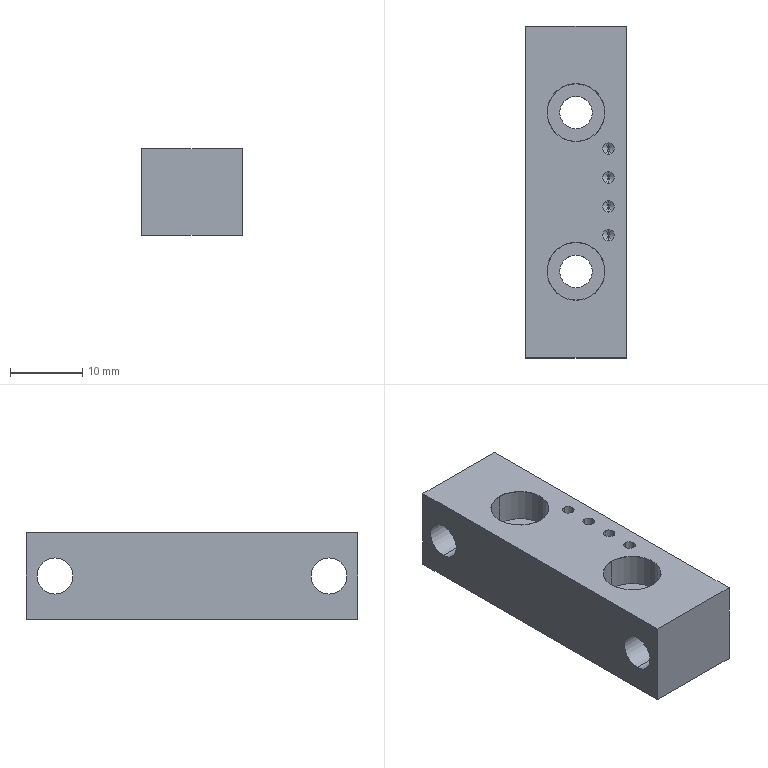Part | NX | features M2 螺纹孔1 2 | 1 solid | 40 faces | box 14 x 46 x 12 mm | volume 6437 mm3 | cylinder 20 | cone 12 | plane 8 | commonest cylinder face diameters 1.6 x8 4.5 x4 5 x4 8 x4
STEP:
#1=CARTESIAN_POINT('',(-56.5,97.8,-87.7));
#2=VERTEX_POINT('',#1);
#3=CARTESIAN_POINT('',(-56.5,96.2,-87.7));
#4=VERTEX_POINT('',#3);
#5=CARTESIAN_POINT('',(-56.5,97.,-87.7));
#6=DIRECTION('',(0.,0.,1.));
#7=DIRECTION('',(0.,-1.,0.));
#8=AXIS2_PLACEMENT_3D('',#5,#6,#7);
#9=CIRCLE('',#8,0.8);
#10=EDGE_CURVE('',#2,#4,#9,.T.);
#11=ORIENTED_EDGE('',*,*,#10,.F.);
#12=CARTESIAN_POINT('',(-56.5,97.8,-82.5));
#13=VERTEX_POINT('',#12);
#14=CARTESIAN_POINT('',(-56.5,97.8,-82.5));
#15=DIRECTION('',(0.,0.,1.));
#16=VECTOR('',#15,1000.);
#17=LINE('',#14,#16);
#18=EDGE_CURVE('',#2,#13,#17,.T.);
#19=ORIENTED_EDGE('',*,*,#18,.T.);
#20=CARTESIAN_POINT('',(-56.5,96.2,-82.5));
#21=VERTEX_POINT('',#20);
#22=CARTESIAN_POINT('',(-56.5,97.,-82.5));
#23=DIRECTION('',(0.,0.,1.));
#24=DIRECTION('',(0.,-1.,0.));
#25=AXIS2_PLACEMENT_3D('',#22,#23,#24);
#26=CIRCLE('',#25,0.8);
#27=EDGE_CURVE('',#13,#21,#26,.T.);
#28=ORIENTED_EDGE('',*,*,#27,.T.);
#29=CARTESIAN_POINT('',(-56.5,96.2,-82.5));
#30=DIRECTION('',(0.,0.,1.));
#31=VECTOR('',#30,1000.);
#32=LINE('',#29,#31);
#33=EDGE_CURVE('',#21,#4,#32,.F.);
#34=ORIENTED_EDGE('',*,*,#33,.T.);
#35=EDGE_LOOP('',(#11,#19,#28,#34));
#36=FACE_BOUND('',#35,.T.);
#37=CARTESIAN_POINT('',(-56.5,97.,-82.5));
#38=DIRECTION('',(0.,0.,1.));
#39=DIRECTION('',(0.,1.,0.));
#40=AXIS2_PLACEMENT_3D('',#37,#38,#39);
#41=CYLINDRICAL_SURFACE('',#40,0.8);
#42=ADVANCED_FACE('',(#36),#41,.F.);
#43=CARTESIAN_POINT('',(-56.5,97.,-88.181));
#44=VERTEX_POINT('',#43);
#45=CARTESIAN_POINT('',(-56.5,96.2,-87.7));
#46=DIRECTION('',(0.,-0.8572,0.515));
#47=VECTOR('',#46,1000.);
#48=LINE('',#45,#47);
#49=EDGE_CURVE('',#4,#44,#48,.F.);
#50=ORIENTED_EDGE('',*,*,#49,.T.);
#51=CARTESIAN_POINT('',(-56.5,97.8,-87.7));
#52=DIRECTION('',(0.,0.8572,0.515));
#53=VECTOR('',#52,1000.);
#54=LINE('',#51,#53);
#55=EDGE_CURVE('',#44,#2,#54,.T.);
#56=ORIENTED_EDGE('',*,*,#55,.T.);
#57=ORIENTED_EDGE('',*,*,#10,.T.);
#58=EDGE_LOOP('',(#50,#56,#57));
#59=FACE_BOUND('',#58,.T.);
#60=CARTESIAN_POINT('',(-56.5,97.,-87.7));
#61=DIRECTION('',(0.,0.,1.));
#62=DIRECTION('',(0.,1.,0.));
#63=AXIS2_PLACEMENT_3D('',#60,#61,#62);
#64=CONICAL_SURFACE('',#63,0.8,1.03);
#65=ADVANCED_FACE('',(#59),#64,.F.);
#66=CARTESIAN_POINT('',(-56.5,93.8,-87.7));
#67=VERTEX_POINT('',#66);
#68=CARTESIAN_POINT('',(-56.5,92.2,-87.7));
#69=VERTEX_POINT('',#68);
#70=CARTESIAN_POINT('',(-56.5,93.,-87.7));
#71=DIRECTION('',(0.,0.,1.));
#72=DIRECTION('',(0.,-1.,0.));
#73=AXIS2_PLACEMENT_3D('',#70,#71,#72);
#74=CIRCLE('',#73,0.8);
#75=EDGE_CURVE('',#67,#69,#74,.T.);
#76=ORIENTED_EDGE('',*,*,#75,.F.);
#77=CARTESIAN_POINT('',(-56.5,93.8,-82.5));
#78=VERTEX_POINT('',#77);
#79=CARTESIAN_POINT('',(-56.5,93.8,-82.5));
#80=DIRECTION('',(0.,0.,1.));
#81=VECTOR('',#80,1000.);
#82=LINE('',#79,#81);
#83=EDGE_CURVE('',#67,#78,#82,.T.);
#84=ORIENTED_EDGE('',*,*,#83,.T.);
#85=CARTESIAN_POINT('',(-56.5,92.2,-82.5));
#86=VERTEX_POINT('',#85);
#87=CARTESIAN_POINT('',(-56.5,93.,-82.5));
#88=DIRECTION('',(0.,0.,1.));
#89=DIRECTION('',(0.,-1.,0.));
#90=AXIS2_PLACEMENT_3D('',#87,#88,#89);
#91=CIRCLE('',#90,0.8);
#92=EDGE_CURVE('',#78,#86,#91,.T.);
#93=ORIENTED_EDGE('',*,*,#92,.T.);
#94=CARTESIAN_POINT('',(-56.5,92.2,-82.5));
#95=DIRECTION('',(0.,0.,1.));
#96=VECTOR('',#95,1000.);
#97=LINE('',#94,#96);
#98=EDGE_CURVE('',#86,#69,#97,.F.);
#99=ORIENTED_EDGE('',*,*,#98,.T.);
#100=EDGE_LOOP('',(#76,#84,#93,#99));
#101=FACE_BOUND('',#100,.T.);
#102=CARTESIAN_POINT('',(-56.5,93.,-82.5));
#103=DIRECTION('',(0.,0.,1.));
#104=DIRECTION('',(0.,1.,0.));
#105=AXIS2_PLACEMENT_3D('',#102,#103,#104);
#106=CYLINDRICAL_SURFACE('',#105,0.8);
#107=ADVANCED_FACE('',(#101),#106,.F.);
#108=CARTESIAN_POINT('',(-56.5,93.,-88.181));
#109=VERTEX_POINT('',#108);
#110=CARTESIAN_POINT('',(-56.5,92.2,-87.7));
#111=DIRECTION('',(0.,-0.8572,0.515));
#112=VECTOR('',#111,1000.);
#113=LINE('',#110,#112);
#114=EDGE_CURVE('',#109,#69,#113,.T.);
#115=ORIENTED_EDGE('',*,*,#114,.F.);
#116=CARTESIAN_POINT('',(-56.5,93.8,-87.7));
#117=DIRECTION('',(0.,0.8572,0.515));
#118=VECTOR('',#117,1000.);
#119=LINE('',#116,#118);
#120=EDGE_CURVE('',#67,#109,#119,.F.);
#121=ORIENTED_EDGE('',*,*,#120,.F.);
#122=ORIENTED_EDGE('',*,*,#75,.T.);
#123=EDGE_LOOP('',(#115,#121,#122));
#124=FACE_BOUND('',#123,.T.);
#125=CARTESIAN_POINT('',(-56.5,93.,-87.7));
#126=DIRECTION('',(0.,0.,1.));
#127=DIRECTION('',(0.,1.,0.));
#128=AXIS2_PLACEMENT_3D('',#125,#126,#127);
#129=CONICAL_SURFACE('',#128,0.8,1.03);
#130=ADVANCED_FACE('',(#124),#129,.F.);
#131=CARTESIAN_POINT('',(-56.5,105.8,-87.7));
#132=VERTEX_POINT('',#131);
#133=CARTESIAN_POINT('',(-56.5,104.2,-87.7));
#134=VERTEX_POINT('',#133);
#135=CARTESIAN_POINT('',(-56.5,105.,-87.7));
#136=DIRECTION('',(0.,0.,1.));
#137=DIRECTION('',(0.,-1.,0.));
#138=AXIS2_PLACEMENT_3D('',#135,#136,#137);
#139=CIRCLE('',#138,0.8);
#140=EDGE_CURVE('',#132,#134,#139,.T.);
#141=ORIENTED_EDGE('',*,*,#140,.F.);
#142=CARTESIAN_POINT('',(-56.5,105.8,-82.5));
#143=VERTEX_POINT('',#142);
#144=CARTESIAN_POINT('',(-56.5,105.8,-82.5));
#145=DIRECTION('',(0.,0.,1.));
#146=VECTOR('',#145,1000.);
#147=LINE('',#144,#146);
#148=EDGE_CURVE('',#143,#132,#147,.F.);
#149=ORIENTED_EDGE('',*,*,#148,.F.);
#150=CARTESIAN_POINT('',(-56.5,104.2,-82.5));
#151=VERTEX_POINT('',#150);
#152=CARTESIAN_POINT('',(-56.5,105.,-82.5));
#153=DIRECTION('',(0.,0.,1.));
#154=DIRECTION('',(0.,-1.,0.));
#155=AXIS2_PLACEMENT_3D('',#152,#153,#154);
#156=CIRCLE('',#155,0.8);
#157=EDGE_CURVE('',#143,#151,#156,.T.);
#158=ORIENTED_EDGE('',*,*,#157,.T.);
#159=CARTESIAN_POINT('',(-56.5,104.2,-82.5));
#160=DIRECTION('',(0.,0.,1.));
#161=VECTOR('',#160,1000.);
#162=LINE('',#159,#161);
#163=EDGE_CURVE('',#134,#151,#162,.T.);
#164=ORIENTED_EDGE('',*,*,#163,.F.);
#165=EDGE_LOOP('',(#141,#149,#158,#164));
#166=FACE_BOUND('',#165,.T.);
#167=CARTESIAN_POINT('',(-56.5,105.,-82.5));
#168=DIRECTION('',(0.,0.,1.));
#169=DIRECTION('',(0.,1.,0.));
#170=AXIS2_PLACEMENT_3D('',#167,#168,#169);
#171=CYLINDRICAL_SURFACE('',#170,0.8);
#172=ADVANCED_FACE('',(#166),#171,.F.);
#173=CARTESIAN_POINT('',(-56.5,105.,-88.181));
#174=VERTEX_POINT('',#173);
#175=CARTESIAN_POINT('',(-56.5,104.2,-87.7));
#176=DIRECTION('',(0.,-0.8572,0.515));
#177=VECTOR('',#176,1000.);
#178=LINE('',#175,#177);
#179=EDGE_CURVE('',#174,#134,#178,.T.);
#180=ORIENTED_EDGE('',*,*,#179,.F.);
#181=CARTESIAN_POINT('',(-56.5,105.8,-87.7));
#182=DIRECTION('',(0.,0.8572,0.515));
#183=VECTOR('',#182,1000.);
#184=LINE('',#181,#183);
#185=EDGE_CURVE('',#132,#174,#184,.F.);
#186=ORIENTED_EDGE('',*,*,#185,.F.);
#187=ORIENTED_EDGE('',*,*,#140,.T.);
#188=EDGE_LOOP('',(#180,#186,#187));
#189=FACE_BOUND('',#188,.T.);
#190=CARTESIAN_POINT('',(-56.5,105.,-87.7));
#191=DIRECTION('',(0.,0.,1.));
#192=DIRECTION('',(0.,1.,0.));
#193=AXIS2_PLACEMENT_3D('',#190,#191,#192);
#194=CONICAL_SURFACE('',#193,0.8,1.03);
#195=ADVANCED_FACE('',(#189),#194,.F.);
#196=CARTESIAN_POINT('',(-56.5,101.8,-87.7));
#197=VERTEX_POINT('',#196);
#198=CARTESIAN_POINT('',(-56.5,100.2,-87.7));
#199=VERTEX_POINT('',#198);
#200=CARTESIAN_POINT('',(-56.5,101.,-87.7));
#201=DIRECTION('',(0.,0.,1.));
#202=DIRECTION('',(0.,-1.,0.));
#203=AXIS2_PLACEMENT_3D('',#200,#201,#202);
#204=CIRCLE('',#203,0.8);
#205=EDGE_CURVE('',#197,#199,#204,.T.);
#206=ORIENTED_EDGE('',*,*,#205,.F.);
#207=CARTESIAN_POINT('',(-56.5,101.8,-82.5));
#208=VERTEX_POINT('',#207);
#209=CARTESIAN_POINT('',(-56.5,101.8,-82.5));
#210=DIRECTION('',(0.,0.,1.));
#211=VECTOR('',#210,1000.);
#212=LINE('',#209,#211);
#213=EDGE_CURVE('',#197,#208,#212,.T.);
#214=ORIENTED_EDGE('',*,*,#213,.T.);
#215=CARTESIAN_POINT('',(-56.5,100.2,-82.5));
#216=VERTEX_POINT('',#215);
#217=CARTESIAN_POINT('',(-56.5,101.,-82.5));
#218=DIRECTION('',(0.,0.,1.));
#219=DIRECTION('',(0.,-1.,0.));
#220=AXIS2_PLACEMENT_3D('',#217,#218,#219);
#221=CIRCLE('',#220,0.8);
#222=EDGE_CURVE('',#208,#216,#221,.T.);
#223=ORIENTED_EDGE('',*,*,#222,.T.);
#224=CARTESIAN_POINT('',(-56.5,100.2,-82.5));
#225=DIRECTION('',(0.,0.,1.));
#226=VECTOR('',#225,1000.);
#227=LINE('',#224,#226);
#228=EDGE_CURVE('',#216,#199,#227,.F.);
#229=ORIENTED_EDGE('',*,*,#228,.T.);
#230=EDGE_LOOP('',(#206,#214,#223,#229));
#231=FACE_BOUND('',#230,.T.);
#232=CARTESIAN_POINT('',(-56.5,101.,-82.5));
#233=DIRECTION('',(0.,0.,1.));
#234=DIRECTION('',(0.,1.,0.));
#235=AXIS2_PLACEMENT_3D('',#232,#233,#234);
#236=CYLINDRICAL_SURFACE('',#235,0.8);
#237=ADVANCED_FACE('',(#231),#236,.F.);
#238=CARTESIAN_POINT('',(-56.5,101.,-88.181));
#239=VERTEX_POINT('',#238);
#240=CARTESIAN_POINT('',(-56.5,100.2,-87.7));
#241=DIRECTION('',(0.,-0.8572,0.515));
#242=VECTOR('',#241,1000.);
#243=LINE('',#240,#242);
#244=EDGE_CURVE('',#199,#239,#243,.F.);
#245=ORIENTED_EDGE('',*,*,#244,.T.);
#246=CARTESIAN_POINT('',(-56.5,101.8,-87.7));
#247=DIRECTION('',(0.,0.8572,0.515));
#248=VECTOR('',#247,1000.);
#249=LINE('',#246,#248);
#250=EDGE_CURVE('',#239,#197,#249,.T.);
#251=ORIENTED_EDGE('',*,*,#250,.T.);
#252=ORIENTED_EDGE('',*,*,#205,.T.);
#253=EDGE_LOOP('',(#245,#251,#252));
#254=FACE_BOUND('',#253,.T.);
#255=CARTESIAN_POINT('',(-56.5,101.,-87.7));
#256=DIRECTION('',(0.,0.,1.));
#257=DIRECTION('',(0.,1.,0.));
#258=AXIS2_PLACEMENT_3D('',#255,#256,#257);
#259=CONICAL_SURFACE('',#258,0.8,1.03);
#260=ADVANCED_FACE('',(#254),#259,.F.);
#261=CARTESIAN_POINT('',(-54.,80.,-86.));
#262=VERTEX_POINT('',#261);
#263=CARTESIAN_POINT('',(-54.,80.,-91.));
#264=VERTEX_POINT('',#263);
#265=CARTESIAN_POINT('',(-54.,80.,-88.5));
#266=DIRECTION('',(-1.,0.,0.));
#267=DIRECTION('',(0.,0.,-1.));
#268=AXIS2_PLACEMENT_3D('',#265,#266,#267);
#269=CIRCLE('',#268,2.5);
#270=EDGE_CURVE('',#262,#264,#269,.T.);
#271=ORIENTED_EDGE('',*,*,#270,.F.);
#272=CARTESIAN_POINT('',(-68.,80.,-86.));
#273=VERTEX_POINT('',#272);
#274=CARTESIAN_POINT('',(-68.,80.,-86.));
#275=DIRECTION('',(-1.,0.,0.));
#276=VECTOR('',#275,1000.);
#277=LINE('',#274,#276);
#278=EDGE_CURVE('',#262,#273,#277,.T.);
#279=ORIENTED_EDGE('',*,*,#278,.T.);
#280=CARTESIAN_POINT('',(-68.,80.,-91.));
#281=VERTEX_POINT('',#280);
#282=CARTESIAN_POINT('',(-68.,80.,-88.5));
#283=DIRECTION('',(-1.,0.,0.));
#284=DIRECTION('',(0.,0.,-1.));
#285=AXIS2_PLACEMENT_3D('',#282,#283,#284);
#286=CIRCLE('',#285,2.5);
#287=EDGE_CURVE('',#273,#281,#286,.T.);
#288=ORIENTED_EDGE('',*,*,#287,.T.);
#289=CARTESIAN_POINT('',(-68.,80.,-91.));
#290=DIRECTION('',(-1.,0.,0.));
#291=VECTOR('',#290,1000.);
#292=LINE('',#289,#291);
#293=EDGE_CURVE('',#281,#264,#292,.F.);
#294=ORIENTED_EDGE('',*,*,#293,.T.);
#295=EDGE_LOOP('',(#271,#279,#288,#294));
#296=FACE_BOUND('',#295,.T.);
#297=CARTESIAN_POINT('',(-68.,80.,-88.5));
#298=DIRECTION('',(-1.,0.,0.));
#299=DIRECTION('',(0.,0.,1.));
#300=AXIS2_PLACEMENT_3D('',#297,#298,#299);
#301=CYLINDRICAL_SURFACE('',#300,2.5);
#302=ADVANCED_FACE('',(#296),#301,.F.);
#303=CARTESIAN_POINT('',(-54.,118.,-86.));
#304=VERTEX_POINT('',#303);
#305=CARTESIAN_POINT('',(-54.,118.,-91.));
#306=VERTEX_POINT('',#305);
#307=CARTESIAN_POINT('',(-54.,118.,-88.5));
#308=DIRECTION('',(-1.,0.,0.));
#309=DIRECTION('',(0.,0.,-1.));
#310=AXIS2_PLACEMENT_3D('',#307,#308,#309);
#311=CIRCLE('',#310,2.5);
#312=EDGE_CURVE('',#304,#306,#311,.T.);
#313=ORIENTED_EDGE('',*,*,#312,.F.);
#314=CARTESIAN_POINT('',(-68.,118.,-86.));
#315=VERTEX_POINT('',#314);
#316=CARTESIAN_POINT('',(-68.,118.,-86.));
#317=DIRECTION('',(-1.,0.,0.));
#318=VECTOR('',#317,1000.);
#319=LINE('',#316,#318);
#320=EDGE_CURVE('',#304,#315,#319,.T.);
#321=ORIENTED_EDGE('',*,*,#320,.T.);
#322=CARTESIAN_POINT('',(-68.,118.,-91.));
#323=VERTEX_POINT('',#322);
#324=CARTESIAN_POINT('',(-68.,118.,-88.5));
#325=DIRECTION('',(-1.,0.,0.));
#326=DIRECTION('',(0.,0.,-1.));
#327=AXIS2_PLACEMENT_3D('',#324,#325,#326);
#328=CIRCLE('',#327,2.5);
#329=EDGE_CURVE('',#315,#323,#328,.T.);
#330=ORIENTED_EDGE('',*,*,#329,.T.);
#331=CARTESIAN_POINT('',(-68.,118.,-91.));
#332=DIRECTION('',(-1.,0.,0.));
#333=VECTOR('',#332,1000.);
#334=LINE('',#331,#333);
#335=EDGE_CURVE('',#323,#306,#334,.F.);
#336=ORIENTED_EDGE('',*,*,#335,.T.);
#337=EDGE_LOOP('',(#313,#321,#330,#336));
#338=FACE_BOUND('',#337,.T.);
#339=CARTESIAN_POINT('',(-68.,118.,-88.5));
#340=DIRECTION('',(-1.,0.,0.));
#341=DIRECTION('',(0.,0.,1.));
#342=AXIS2_PLACEMENT_3D('',#339,#340,#341);
#343=CYLINDRICAL_SURFACE('',#342,2.5);
#344=ADVANCED_FACE('',(#338),#343,.F.);
#345=CARTESIAN_POINT('',(-61.,92.,-82.525));
#346=VERTEX_POINT('',#345);
#347=CARTESIAN_POINT('',(-61.,84.,-82.525));
#348=VERTEX_POINT('',#347);
#349=CARTESIAN_POINT('',(-61.,88.,-82.525));
#350=DIRECTION('',(0.,0.,1.));
#351=DIRECTION('',(0.,-1.,0.));
#352=AXIS2_PLACEMENT_3D('',#349,#350,#351);
#353=CIRCLE('',#352,4.);
#354=EDGE_CURVE('',#346,#348,#353,.T.);
#355=ORIENTED_EDGE('',*,*,#354,.F.);
#356=CARTESIAN_POINT('',(-61.,92.025,-82.5));
#357=VERTEX_POINT('',#356);
#358=CARTESIAN_POINT('',(-61.,92.025,-82.5));
#359=DIRECTION('',(0.,0.7071,0.7071));
#360=VECTOR('',#359,1000.);
#361=LINE('',#358,#360);
#362=EDGE_CURVE('',#346,#357,#361,.T.);
#363=ORIENTED_EDGE('',*,*,#362,.T.);
#364=CARTESIAN_POINT('',(-61.,83.975,-82.5));
#365=VERTEX_POINT('',#364);
#366=CARTESIAN_POINT('',(-61.,88.,-82.5));
#367=DIRECTION('',(0.,0.,1.));
#368=DIRECTION('',(0.,-1.,0.));
#369=AXIS2_PLACEMENT_3D('',#366,#367,#368);
#370=CIRCLE('',#369,4.025);
#371=EDGE_CURVE('',#357,#365,#370,.T.);
#372=ORIENTED_EDGE('',*,*,#371,.T.);
#373=CARTESIAN_POINT('',(-61.,83.975,-82.5));
#374=DIRECTION('',(0.,-0.7071,0.7071));
#375=VECTOR('',#374,1000.);
#376=LINE('',#373,#375);
#377=EDGE_CURVE('',#365,#348,#376,.F.);
#378=ORIENTED_EDGE('',*,*,#377,.T.);
#379=EDGE_LOOP('',(#355,#363,#372,#378));
#380=FACE_BOUND('',#379,.T.);
#381=CARTESIAN_POINT('',(-61.,88.,-82.5));
#382=DIRECTION('',(0.,0.,1.));
#383=DIRECTION('',(0.,1.,0.));
#384=AXIS2_PLACEMENT_3D('',#381,#382,#383);
#385=CONICAL_SURFACE('',#384,4.025,0.7854);
#386=ADVANCED_FACE('',(#380),#385,.F.);
#387=CARTESIAN_POINT('',(-61.,92.,-87.1));
#388=VERTEX_POINT('',#387);
#389=CARTESIAN_POINT('',(-61.,84.,-87.1));
#390=VERTEX_POINT('',#389);
#391=CARTESIAN_POINT('',(-61.,88.,-87.1));
#392=DIRECTION('',(0.,0.,1.));
#393=DIRECTION('',(0.,-1.,0.));
#394=AXIS2_PLACEMENT_3D('',#391,#392,#393);
#395=CIRCLE('',#394,4.);
#396=EDGE_CURVE('',#388,#390,#395,.T.);
#397=ORIENTED_EDGE('',*,*,#396,.F.);
#398=CARTESIAN_POINT('',(-61.,92.,-82.5));
#399=DIRECTION('',(0.,0.,1.));
#400=VECTOR('',#399,1000.);
#401=LINE('',#398,#400);
#402=EDGE_CURVE('',#388,#346,#401,.T.);
#403=ORIENTED_EDGE('',*,*,#402,.T.);
#404=ORIENTED_EDGE('',*,*,#354,.T.);
#405=CARTESIAN_POINT('',(-61.,84.,-82.5));
#406=DIRECTION('',(0.,0.,1.));
#407=VECTOR('',#406,1000.);
#408=LINE('',#405,#407);
#409=EDGE_CURVE('',#348,#390,#408,.F.);
#410=ORIENTED_EDGE('',*,*,#409,.T.);
#411=EDGE_LOOP('',(#397,#403,#404,#410));
#412=FACE_BOUND('',#411,.T.);
#413=CARTESIAN_POINT('',(-61.,88.,-82.5));
#414=DIRECTION('',(0.,0.,1.));
#415=DIRECTION('',(0.,1.,0.));
#416=AXIS2_PLACEMENT_3D('',#413,#414,#415);
#417=CYLINDRICAL_SURFACE('',#416,4.);
#418=ADVANCED_FACE('',(#412),#417,.F.);
#419=CARTESIAN_POINT('',(-61.,90.25,-94.5));
#420=VERTEX_POINT('',#419);
#421=CARTESIAN_POINT('',(-61.,85.75,-94.5));
#422=VERTEX_POINT('',#421);
#423=CARTESIAN_POINT('',(-61.,88.,-94.5));
#424=DIRECTION('',(0.,0.,1.));
#425=DIRECTION('',(0.,-1.,0.));
#426=AXIS2_PLACEMENT_3D('',#423,#424,#425);
#427=CIRCLE('',#426,2.25);
#428=EDGE_CURVE('',#420,#422,#427,.T.);
#429=ORIENTED_EDGE('',*,*,#428,.F.);
#430=CARTESIAN_POINT('',(-61.,90.25,-87.1));
#431=VERTEX_POINT('',#430);
#432=CARTESIAN_POINT('',(-61.,90.25,-82.5));
#433=DIRECTION('',(0.,0.,1.));
#434=VECTOR('',#433,1000.);
#435=LINE('',#432,#434);
#436=EDGE_CURVE('',#431,#420,#435,.F.);
#437=ORIENTED_EDGE('',*,*,#436,.F.);
#438=CARTESIAN_POINT('',(-61.,85.75,-87.1));
#439=VERTEX_POINT('',#438);
#440=CARTESIAN_POINT('',(-61.,88.,-87.1));
#441=DIRECTION('',(0.,0.,1.));
#442=DIRECTION('',(0.,-1.,0.));
#443=AXIS2_PLACEMENT_3D('',#440,#441,#442);
#444=CIRCLE('',#443,2.25);
#445=EDGE_CURVE('',#431,#439,#444,.T.);
#446=ORIENTED_EDGE('',*,*,#445,.T.);
#447=CARTESIAN_POINT('',(-61.,85.75,-82.5));
#448=DIRECTION('',(0.,0.,1.));
#449=VECTOR('',#448,1000.);
#450=LINE('',#447,#449);
#451=EDGE_CURVE('',#422,#439,#450,.T.);
#452=ORIENTED_EDGE('',*,*,#451,.F.);
#453=EDGE_LOOP('',(#429,#437,#446,#452));
#454=FACE_BOUND('',#453,.T.);
#455=CARTESIAN_POINT('',(-61.,88.,-82.5));
#456=DIRECTION('',(0.,0.,1.));
#457=DIRECTION('',(0.,1.,0.));
#458=AXIS2_PLACEMENT_3D('',#455,#456,#457);
#459=CYLINDRICAL_SURFACE('',#458,2.25);
#460=ADVANCED_FACE('',(#454),#459,.F.);
#461=CARTESIAN_POINT('',(-61.,114.,-82.525));
#462=VERTEX_POINT('',#461);
#463=CARTESIAN_POINT('',(-61.,106.,-82.525));
#464=VERTEX_POINT('',#463);
#465=CARTESIAN_POINT('',(-61.,110.,-82.525));
#466=DIRECTION('',(0.,0.,1.));
#467=DIRECTION('',(0.,-1.,0.));
#468=AXIS2_PLACEMENT_3D('',#465,#466,#467);
#469=CIRCLE('',#468,4.);
#470=EDGE_CURVE('',#462,#464,#469,.T.);
#471=ORIENTED_EDGE('',*,*,#470,.F.);
#472=CARTESIAN_POINT('',(-61.,114.025,-82.5));
#473=VERTEX_POINT('',#472);
#474=CARTESIAN_POINT('',(-61.,114.025,-82.5));
#475=DIRECTION('',(0.,0.7071,0.7071));
#476=VECTOR('',#475,1000.);
#477=LINE('',#474,#476);
#478=EDGE_CURVE('',#473,#462,#477,.F.);
#479=ORIENTED_EDGE('',*,*,#478,.F.);
#480=CARTESIAN_POINT('',(-61.,105.975,-82.5));
#481=VERTEX_POINT('',#480);
#482=CARTESIAN_POINT('',(-61.,110.,-82.5));
#483=DIRECTION('',(0.,0.,1.));
#484=DIRECTION('',(0.,-1.,0.));
#485=AXIS2_PLACEMENT_3D('',#482,#483,#484);
#486=CIRCLE('',#485,4.025);
#487=EDGE_CURVE('',#473,#481,#486,.T.);
#488=ORIENTED_EDGE('',*,*,#487,.T.);
#489=CARTESIAN_POINT('',(-61.,105.975,-82.5));
#490=DIRECTION('',(0.,-0.7071,0.7071));
#491=VECTOR('',#490,1000.);
#492=LINE('',#489,#491);
#493=EDGE_CURVE('',#464,#481,#492,.T.);
#494=ORIENTED_EDGE('',*,*,#493,.F.);
#495=EDGE_LOOP('',(#471,#479,#488,#494));
#496=FACE_BOUND('',#495,.T.);
#497=CARTESIAN_POINT('',(-61.,110.,-82.5));
#498=DIRECTION('',(0.,0.,1.));
#499=DIRECTION('',(0.,1.,0.));
#500=AXIS2_PLACEMENT_3D('',#497,#498,#499);
#501=CONICAL_SURFACE('',#500,4.025,0.7854);
#502=ADVANCED_FACE('',(#496),#501,.F.);
#503=CARTESIAN_POINT('',(-61.,114.,-87.1));
#504=VERTEX_POINT('',#503);
#505=CARTESIAN_POINT('',(-61.,106.,-87.1));
#506=VERTEX_POINT('',#505);
#507=CARTESIAN_POINT('',(-61.,110.,-87.1));
#508=DIRECTION('',(0.,0.,1.));
#509=DIRECTION('',(0.,-1.,0.));
#510=AXIS2_PLACEMENT_3D('',#507,#508,#509);
#511=CIRCLE('',#510,4.);
#512=EDGE_CURVE('',#504,#506,#511,.T.);
#513=ORIENTED_EDGE('',*,*,#512,.F.);
#514=CARTESIAN_POINT('',(-61.,114.,-82.5));
#515=DIRECTION('',(0.,0.,1.));
#516=VECTOR('',#515,1000.);
#517=LINE('',#514,#516);
#518=EDGE_CURVE('',#462,#504,#517,.F.);
#519=ORIENTED_EDGE('',*,*,#518,.F.);
#520=ORIENTED_EDGE('',*,*,#470,.T.);
#521=CARTESIAN_POINT('',(-61.,106.,-82.5));
#522=DIRECTION('',(0.,0.,1.));
#523=VECTOR('',#522,1000.);
#524=LINE('',#521,#523);
#525=EDGE_CURVE('',#506,#464,#524,.T.);
#526=ORIENTED_EDGE('',*,*,#525,.F.);
#527=EDGE_LOOP('',(#513,#519,#520,#526));
#528=FACE_BOUND('',#527,.T.);
#529=CARTESIAN_POINT('',(-61.,110.,-82.5));
#530=DIRECTION('',(0.,0.,1.));
#531=DIRECTION('',(0.,1.,0.));
#532=AXIS2_PLACEMENT_3D('',#529,#530,#531);
#533=CYLINDRICAL_SURFACE('',#532,4.);
#534=ADVANCED_FACE('',(#528),#533,.F.);
#535=CARTESIAN_POINT('',(-61.,112.25,-94.5));
#536=VERTEX_POINT('',#535);
#537=CARTESIAN_POINT('',(-61.,107.75,-94.5));
#538=VERTEX_POINT('',#537);
#539=CARTESIAN_POINT('',(-61.,110.,-94.5));
#540=DIRECTION('',(0.,0.,1.));
#541=DIRECTION('',(0.,-1.,0.));
#542=AXIS2_PLACEMENT_3D('',#539,#540,#541);
#543=CIRCLE('',#542,2.25);
#544=EDGE_CURVE('',#536,#538,#543,.T.);
#545=ORIENTED_EDGE('',*,*,#544,.F.);
#546=CARTESIAN_POINT('',(-61.,112.25,-87.1));
#547=VERTEX_POINT('',#546);
#548=CARTESIAN_POINT('',(-61.,112.25,-82.5));
#549=DIRECTION('',(0.,0.,1.));
#550=VECTOR('',#549,1000.);
#551=LINE('',#548,#550);
#552=EDGE_CURVE('',#536,#547,#551,.T.);
#553=ORIENTED_EDGE('',*,*,#552,.T.);
#554=CARTESIAN_POINT('',(-61.,107.75,-87.1));
#555=VERTEX_POINT('',#554);
#556=CARTESIAN_POINT('',(-61.,110.,-87.1));
#557=DIRECTION('',(0.,0.,1.));
#558=DIRECTION('',(0.,-1.,0.));
#559=AXIS2_PLACEMENT_3D('',#556,#557,#558);
#560=CIRCLE('',#559,2.25);
#561=EDGE_CURVE('',#547,#555,#560,.T.);
#562=ORIENTED_EDGE('',*,*,#561,.T.);
#563=CARTESIAN_POINT('',(-61.,107.75,-82.5));
#564=DIRECTION('',(0.,0.,1.));
#565=VECTOR('',#564,1000.);
#566=LINE('',#563,#565);
#567=EDGE_CURVE('',#555,#538,#566,.F.);
#568=ORIENTED_EDGE('',*,*,#567,.T.);
#569=EDGE_LOOP('',(#545,#553,#562,#568));
#570=FACE_BOUND('',#569,.T.);
#571=CARTESIAN_POINT('',(-61.,110.,-82.5));
#572=DIRECTION('',(0.,0.,1.));
#573=DIRECTION('',(0.,1.,0.));
#574=AXIS2_PLACEMENT_3D('',#571,#572,#573);
#575=CYLINDRICAL_SURFACE('',#574,2.25);
#576=ADVANCED_FACE('',(#570),#575,.F.);
#577=CARTESIAN_POINT('',(-68.,76.,-94.5));
#578=VERTEX_POINT('',#577);
#579=CARTESIAN_POINT('',(-54.,76.,-94.5));
#580=VERTEX_POINT('',#579);
#581=CARTESIAN_POINT('',(-54.,76.,-94.5));
#582=DIRECTION('',(1.,0.,0.));
#583=VECTOR('',#582,1000.);
#584=LINE('',#581,#583);
#585=EDGE_CURVE('',#578,#580,#584,.T.);
#586=ORIENTED_EDGE('',*,*,#585,.T.);
#587=CARTESIAN_POINT('',(-54.,76.,-82.5));
#588=VERTEX_POINT('',#587);
#589=CARTESIAN_POINT('',(-54.,76.,-82.5));
#590=DIRECTION('',(0.,0.,-1.));
#591=VECTOR('',#590,1000.);
#592=LINE('',#589,#591);
#593=EDGE_CURVE('',#588,#580,#592,.T.);
#594=ORIENTED_EDGE('',*,*,#593,.F.);
#595=CARTESIAN_POINT('',(-68.,76.,-82.5));
#596=VERTEX_POINT('',#595);
#597=CARTESIAN_POINT('',(-54.,76.,-82.5));
#598=DIRECTION('',(1.,0.,0.));
#599=VECTOR('',#598,1000.);
#600=LINE('',#597,#599);
#601=EDGE_CURVE('',#596,#588,#600,.T.);
#602=ORIENTED_EDGE('',*,*,#601,.F.);
#603=CARTESIAN_POINT('',(-68.,76.,-82.5));
#604=DIRECTION('',(0.,0.,-1.));
#605=VECTOR('',#604,1000.);
#606=LINE('',#603,#605);
#607=EDGE_CURVE('',#596,#578,#606,.T.);
#608=ORIENTED_EDGE('',*,*,#607,.T.);
#609=EDGE_LOOP('',(#586,#594,#602,#608));
#610=FACE_BOUND('',#609,.T.);
#611=CARTESIAN_POINT('',(-54.,76.,-82.5));
#612=DIRECTION('',(0.,1.,0.));
#613=DIRECTION('',(0.,0.,-1.));
#614=AXIS2_PLACEMENT_3D('',#611,#612,#613);
#615=PLANE('',#614);
#616=ADVANCED_FACE('',(#610),#615,.F.);
#617=CARTESIAN_POINT('',(-54.,80.,-88.5));
#618=DIRECTION('',(-1.,0.,0.));
#619=DIRECTION('',(0.,0.,-1.));
#620=AXIS2_PLACEMENT_3D('',#617,#618,#619);
#621=CIRCLE('',#620,2.5);
#622=EDGE_CURVE('',#264,#262,#621,.T.);
#623=ORIENTED_EDGE('',*,*,#622,.T.);
#624=ORIENTED_EDGE('',*,*,#270,.T.);
#625=EDGE_LOOP('',(#623,#624));
#626=FACE_BOUND('',#625,.T.);
#627=CARTESIAN_POINT('',(-54.,118.,-88.5));
#628=DIRECTION('',(-1.,0.,0.));
#629=DIRECTION('',(0.,0.,-1.));
#630=AXIS2_PLACEMENT_3D('',#627,#628,#629);
#631=CIRCLE('',#630,2.5);
#632=EDGE_CURVE('',#306,#304,#631,.T.);
#633=ORIENTED_EDGE('',*,*,#632,.T.);
#634=ORIENTED_EDGE('',*,*,#312,.T.);
#635=EDGE_LOOP('',(#633,#634));
#636=FACE_BOUND('',#635,.T.);
#637=CARTESIAN_POINT('',(-54.,122.,-94.5));
#638=VERTEX_POINT('',#637);
#639=CARTESIAN_POINT('',(-54.,122.,-94.5));
#640=DIRECTION('',(0.,1.,0.));
#641=VECTOR('',#640,1000.);
#642=LINE('',#639,#641);
#643=EDGE_CURVE('',#580,#638,#642,.T.);
#644=ORIENTED_EDGE('',*,*,#643,.T.);
#645=CARTESIAN_POINT('',(-54.,122.,-82.5));
#646=VERTEX_POINT('',#645);
#647=CARTESIAN_POINT('',(-54.,122.,-82.5));
#648=DIRECTION('',(0.,0.,-1.));
#649=VECTOR('',#648,1000.);
#650=LINE('',#647,#649);
#651=EDGE_CURVE('',#646,#638,#650,.T.);
#652=ORIENTED_EDGE('',*,*,#651,.F.);
#653=CARTESIAN_POINT('',(-54.,122.,-82.5));
#654=DIRECTION('',(0.,1.,0.));
#655=VECTOR('',#654,1000.);
#656=LINE('',#653,#655);
#657=EDGE_CURVE('',#588,#646,#656,.T.);
#658=ORIENTED_EDGE('',*,*,#657,.F.);
#659=ORIENTED_EDGE('',*,*,#593,.T.);
#660=EDGE_LOOP('',(#644,#652,#658,#659));
#661=FACE_BOUND('',#660,.T.);
#662=CARTESIAN_POINT('',(-54.,122.,-82.5));
#663=DIRECTION('',(-1.,0.,0.));
#664=DIRECTION('',(0.,0.,1.));
#665=AXIS2_PLACEMENT_3D('',#662,#663,#664);
#666=PLANE('',#665);
#667=ADVANCED_FACE('',(#626,#636,#661),#666,.F.);
#668=CARTESIAN_POINT('',(-68.,122.,-94.5));
#669=VERTEX_POINT('',#668);
#670=CARTESIAN_POINT('',(-54.,122.,-94.5));
#671=DIRECTION('',(-1.,0.,0.));
#672=VECTOR('',#671,1000.);
#673=LINE('',#670,#672);
#674=EDGE_CURVE('',#638,#669,#673,.T.);
#675=ORIENTED_EDGE('',*,*,#674,.T.);
#676=CARTESIAN_POINT('',(-68.,122.,-82.5));
#677=VERTEX_POINT('',#676);
#678=CARTESIAN_POINT('',(-68.,122.,-82.5));
#679=DIRECTION('',(0.,0.,-1.));
#680=VECTOR('',#679,1000.);
#681=LINE('',#678,#680);
#682=EDGE_CURVE('',#677,#669,#681,.T.);
#683=ORIENTED_EDGE('',*,*,#682,.F.);
#684=CARTESIAN_POINT('',(-54.,122.,-82.5));
#685=DIRECTION('',(-1.,0.,0.));
#686=VECTOR('',#685,1000.);
#687=LINE('',#684,#686);
#688=EDGE_CURVE('',#646,#677,#687,.T.);
#689=ORIENTED_EDGE('',*,*,#688,.F.);
#690=ORIENTED_EDGE('',*,*,#651,.T.);
#691=EDGE_LOOP('',(#675,#683,#689,#690));
#692=FACE_BOUND('',#691,.T.);
#693=CARTESIAN_POINT('',(-54.,122.,-82.5));
#694=DIRECTION('',(0.,-1.,0.));
#695=DIRECTION('',(0.,0.,1.));
#696=AXIS2_PLACEMENT_3D('',#693,#694,#695);
#697=PLANE('',#696);
#698=ADVANCED_FACE('',(#692),#697,.F.);
#699=CARTESIAN_POINT('',(-68.,80.,-88.5));
#700=DIRECTION('',(-1.,0.,0.));
#701=DIRECTION('',(0.,0.,-1.));
#702=AXIS2_PLACEMENT_3D('',#699,#700,#701);
#703=CIRCLE('',#702,2.5);
#704=EDGE_CURVE('',#281,#273,#703,.T.);
#705=ORIENTED_EDGE('',*,*,#704,.F.);
#706=ORIENTED_EDGE('',*,*,#287,.F.);
#707=EDGE_LOOP('',(#705,#706));
#708=FACE_BOUND('',#707,.T.);
#709=CARTESIAN_POINT('',(-68.,118.,-88.5));
#710=DIRECTION('',(-1.,0.,0.));
#711=DIRECTION('',(0.,0.,-1.));
#712=AXIS2_PLACEMENT_3D('',#709,#710,#711);
#713=CIRCLE('',#712,2.5);
#714=EDGE_CURVE('',#323,#315,#713,.T.);
#715=ORIENTED_EDGE('',*,*,#714,.F.);
#716=ORIENTED_EDGE('',*,*,#329,.F.);
#717=EDGE_LOOP('',(#715,#716));
#718=FACE_BOUND('',#717,.T.);
#719=CARTESIAN_POINT('',(-68.,122.,-94.5));
#720=DIRECTION('',(0.,-1.,0.));
#721=VECTOR('',#720,1000.);
#722=LINE('',#719,#721);
#723=EDGE_CURVE('',#669,#578,#722,.T.);
#724=ORIENTED_EDGE('',*,*,#723,.T.);
#725=ORIENTED_EDGE('',*,*,#607,.F.);
#726=CARTESIAN_POINT('',(-68.,122.,-82.5));
#727=DIRECTION('',(0.,-1.,0.));
#728=VECTOR('',#727,1000.);
#729=LINE('',#726,#728);
#730=EDGE_CURVE('',#677,#596,#729,.T.);
#731=ORIENTED_EDGE('',*,*,#730,.F.);
#732=ORIENTED_EDGE('',*,*,#682,.T.);
#733=EDGE_LOOP('',(#724,#725,#731,#732));
#734=FACE_BOUND('',#733,.T.);
#735=CARTESIAN_POINT('',(-68.,122.,-82.5));
#736=DIRECTION('',(1.,0.,0.));
#737=DIRECTION('',(0.,0.,-1.));
#738=AXIS2_PLACEMENT_3D('',#735,#736,#737);
#739=PLANE('',#738);
#740=ADVANCED_FACE('',(#708,#718,#734),#739,.F.);
#741=CARTESIAN_POINT('',(-56.5,97.,-82.5));
#742=DIRECTION('',(0.,0.,1.));
#743=DIRECTION('',(0.,-1.,0.));
#744=AXIS2_PLACEMENT_3D('',#741,#742,#743);
#745=CIRCLE('',#744,0.8);
#746=EDGE_CURVE('',#21,#13,#745,.T.);
#747=ORIENTED_EDGE('',*,*,#746,.F.);
#748=ORIENTED_EDGE('',*,*,#27,.F.);
#749=EDGE_LOOP('',(#747,#748));
#750=FACE_BOUND('',#749,.T.);
#751=CARTESIAN_POINT('',(-56.5,93.,-82.5));
#752=DIRECTION('',(0.,0.,1.));
#753=DIRECTION('',(0.,-1.,0.));
#754=AXIS2_PLACEMENT_3D('',#751,#752,#753);
#755=CIRCLE('',#754,0.8);
#756=EDGE_CURVE('',#86,#78,#755,.T.);
#757=ORIENTED_EDGE('',*,*,#756,.F.);
#758=ORIENTED_EDGE('',*,*,#92,.F.);
#759=EDGE_LOOP('',(#757,#758));
#760=FACE_BOUND('',#759,.T.);
#761=CARTESIAN_POINT('',(-56.5,105.,-82.5));
#762=DIRECTION('',(0.,0.,1.));
#763=DIRECTION('',(0.,-1.,0.));
#764=AXIS2_PLACEMENT_3D('',#761,#762,#763);
#765=CIRCLE('',#764,0.8);
#766=EDGE_CURVE('',#151,#143,#765,.T.);
#767=ORIENTED_EDGE('',*,*,#766,.F.);
#768=ORIENTED_EDGE('',*,*,#157,.F.);
#769=EDGE_LOOP('',(#767,#768));
#770=FACE_BOUND('',#769,.T.);
#771=CARTESIAN_POINT('',(-56.5,101.,-82.5));
#772=DIRECTION('',(0.,0.,1.));
#773=DIRECTION('',(0.,-1.,0.));
#774=AXIS2_PLACEMENT_3D('',#771,#772,#773);
#775=CIRCLE('',#774,0.8);
#776=EDGE_CURVE('',#216,#208,#775,.T.);
#777=ORIENTED_EDGE('',*,*,#776,.F.);
#778=ORIENTED_EDGE('',*,*,#222,.F.);
#779=EDGE_LOOP('',(#777,#778));
#780=FACE_BOUND('',#779,.T.);
#781=CARTESIAN_POINT('',(-61.,88.,-82.5));
#782=DIRECTION('',(0.,0.,1.));
#783=DIRECTION('',(0.,-1.,0.));
#784=AXIS2_PLACEMENT_3D('',#781,#782,#783);
#785=CIRCLE('',#784,4.025);
#786=EDGE_CURVE('',#365,#357,#785,.T.);
#787=ORIENTED_EDGE('',*,*,#786,.F.);
#788=ORIENTED_EDGE('',*,*,#371,.F.);
#789=EDGE_LOOP('',(#787,#788));
#790=FACE_BOUND('',#789,.T.);
#791=CARTESIAN_POINT('',(-61.,110.,-82.5));
#792=DIRECTION('',(0.,0.,1.));
#793=DIRECTION('',(0.,-1.,0.));
#794=AXIS2_PLACEMENT_3D('',#791,#792,#793);
#795=CIRCLE('',#794,4.025);
#796=EDGE_CURVE('',#481,#473,#795,.T.);
#797=ORIENTED_EDGE('',*,*,#796,.F.);
#798=ORIENTED_EDGE('',*,*,#487,.F.);
#799=EDGE_LOOP('',(#797,#798));
#800=FACE_BOUND('',#799,.T.);
#801=ORIENTED_EDGE('',*,*,#601,.T.);
#802=ORIENTED_EDGE('',*,*,#657,.T.);
#803=ORIENTED_EDGE('',*,*,#688,.T.);
#804=ORIENTED_EDGE('',*,*,#730,.T.);
#805=EDGE_LOOP('',(#801,#802,#803,#804));
#806=FACE_BOUND('',#805,.T.);
#807=CARTESIAN_POINT('',(-61.,99.,-82.5));
#808=DIRECTION('',(0.,0.,1.));
#809=DIRECTION('',(0.,1.,0.));
#810=AXIS2_PLACEMENT_3D('',#807,#808,#809);
#811=PLANE('',#810);
#812=ADVANCED_FACE('',(#750,#760,#770,#780,#790,#800,#806),#811,.T.);
#813=CARTESIAN_POINT('',(-61.,88.,-94.5));
#814=DIRECTION('',(0.,0.,1.));
#815=DIRECTION('',(0.,-1.,0.));
#816=AXIS2_PLACEMENT_3D('',#813,#814,#815);
#817=CIRCLE('',#816,2.25);
#818=EDGE_CURVE('',#422,#420,#817,.T.);
#819=ORIENTED_EDGE('',*,*,#818,.T.);
#820=ORIENTED_EDGE('',*,*,#428,.T.);
#821=EDGE_LOOP('',(#819,#820));
#822=FACE_BOUND('',#821,.T.);
#823=CARTESIAN_POINT('',(-61.,110.,-94.5));
#824=DIRECTION('',(0.,0.,1.));
#825=DIRECTION('',(0.,-1.,0.));
#826=AXIS2_PLACEMENT_3D('',#823,#824,#825);
#827=CIRCLE('',#826,2.25);
#828=EDGE_CURVE('',#538,#536,#827,.T.);
#829=ORIENTED_EDGE('',*,*,#828,.T.);
#830=ORIENTED_EDGE('',*,*,#544,.T.);
#831=EDGE_LOOP('',(#829,#830));
#832=FACE_BOUND('',#831,.T.);
#833=ORIENTED_EDGE('',*,*,#585,.F.);
#834=ORIENTED_EDGE('',*,*,#723,.F.);
#835=ORIENTED_EDGE('',*,*,#674,.F.);
#836=ORIENTED_EDGE('',*,*,#643,.F.);
#837=EDGE_LOOP('',(#833,#834,#835,#836));
#838=FACE_BOUND('',#837,.T.);
#839=CARTESIAN_POINT('',(-61.,99.,-94.5));
#840=DIRECTION('',(0.,0.,1.));
#841=DIRECTION('',(0.,1.,0.));
#842=AXIS2_PLACEMENT_3D('',#839,#840,#841);
#843=PLANE('',#842);
#844=ADVANCED_FACE('',(#822,#832,#838),#843,.F.);
#845=ORIENTED_EDGE('',*,*,#552,.F.);
#846=ORIENTED_EDGE('',*,*,#828,.F.);
#847=ORIENTED_EDGE('',*,*,#567,.F.);
#848=CARTESIAN_POINT('',(-61.,110.,-87.1));
#849=DIRECTION('',(0.,0.,1.));
#850=DIRECTION('',(0.,-1.,0.));
#851=AXIS2_PLACEMENT_3D('',#848,#849,#850);
#852=CIRCLE('',#851,2.25);
#853=EDGE_CURVE('',#555,#547,#852,.T.);
#854=ORIENTED_EDGE('',*,*,#853,.T.);
#855=EDGE_LOOP('',(#845,#846,#847,#854));
#856=FACE_BOUND('',#855,.T.);
#857=CARTESIAN_POINT('',(-61.,110.,-82.5));
#858=DIRECTION('',(0.,0.,1.));
#859=DIRECTION('',(0.,1.,0.));
#860=AXIS2_PLACEMENT_3D('',#857,#858,#859);
#861=CYLINDRICAL_SURFACE('',#860,2.25);
#862=ADVANCED_FACE('',(#856),#861,.F.);
#863=ORIENTED_EDGE('',*,*,#853,.F.);
#864=ORIENTED_EDGE('',*,*,#561,.F.);
#865=EDGE_LOOP('',(#863,#864));
#866=FACE_BOUND('',#865,.T.);
#867=CARTESIAN_POINT('',(-61.,110.,-87.1));
#868=DIRECTION('',(0.,0.,1.));
#869=DIRECTION('',(0.,-1.,0.));
#870=AXIS2_PLACEMENT_3D('',#867,#868,#869);
#871=CIRCLE('',#870,4.);
#872=EDGE_CURVE('',#506,#504,#871,.T.);
#873=ORIENTED_EDGE('',*,*,#872,.T.);
#874=ORIENTED_EDGE('',*,*,#512,.T.);
#875=EDGE_LOOP('',(#873,#874));
#876=FACE_BOUND('',#875,.T.);
#877=CARTESIAN_POINT('',(-61.,106.,-87.1));
#878=DIRECTION('',(0.,0.,-1.));
#879=DIRECTION('',(0.,-1.,0.));
#880=AXIS2_PLACEMENT_3D('',#877,#878,#879);
#881=PLANE('',#880);
#882=ADVANCED_FACE('',(#866,#876),#881,.F.);
#883=ORIENTED_EDGE('',*,*,#518,.T.);
#884=ORIENTED_EDGE('',*,*,#872,.F.);
#885=ORIENTED_EDGE('',*,*,#525,.T.);
#886=CARTESIAN_POINT('',(-61.,110.,-82.525));
#887=DIRECTION('',(0.,0.,1.));
#888=DIRECTION('',(0.,-1.,0.));
#889=AXIS2_PLACEMENT_3D('',#886,#887,#888);
#890=CIRCLE('',#889,4.);
#891=EDGE_CURVE('',#464,#462,#890,.T.);
#892=ORIENTED_EDGE('',*,*,#891,.T.);
#893=EDGE_LOOP('',(#883,#884,#885,#892));
#894=FACE_BOUND('',#893,.T.);
#895=CARTESIAN_POINT('',(-61.,110.,-82.5));
#896=DIRECTION('',(0.,0.,1.));
#897=DIRECTION('',(0.,1.,0.));
#898=AXIS2_PLACEMENT_3D('',#895,#896,#897);
#899=CYLINDRICAL_SURFACE('',#898,4.);
#900=ADVANCED_FACE('',(#894),#899,.F.);
#901=ORIENTED_EDGE('',*,*,#478,.T.);
#902=ORIENTED_EDGE('',*,*,#891,.F.);
#903=ORIENTED_EDGE('',*,*,#493,.T.);
#904=ORIENTED_EDGE('',*,*,#796,.T.);
#905=EDGE_LOOP('',(#901,#902,#903,#904));
#906=FACE_BOUND('',#905,.T.);
#907=CARTESIAN_POINT('',(-61.,110.,-82.5));
#908=DIRECTION('',(0.,0.,1.));
#909=DIRECTION('',(0.,1.,0.));
#910=AXIS2_PLACEMENT_3D('',#907,#908,#909);
#911=CONICAL_SURFACE('',#910,4.025,0.7854);
#912=ADVANCED_FACE('',(#906),#911,.F.);
#913=ORIENTED_EDGE('',*,*,#436,.T.);
#914=ORIENTED_EDGE('',*,*,#818,.F.);
#915=ORIENTED_EDGE('',*,*,#451,.T.);
#916=CARTESIAN_POINT('',(-61.,88.,-87.1));
#917=DIRECTION('',(0.,0.,1.));
#918=DIRECTION('',(0.,-1.,0.));
#919=AXIS2_PLACEMENT_3D('',#916,#917,#918);
#920=CIRCLE('',#919,2.25);
#921=EDGE_CURVE('',#439,#431,#920,.T.);
#922=ORIENTED_EDGE('',*,*,#921,.T.);
#923=EDGE_LOOP('',(#913,#914,#915,#922));
#924=FACE_BOUND('',#923,.T.);
#925=CARTESIAN_POINT('',(-61.,88.,-82.5));
#926=DIRECTION('',(0.,0.,1.));
#927=DIRECTION('',(0.,1.,0.));
#928=AXIS2_PLACEMENT_3D('',#925,#926,#927);
#929=CYLINDRICAL_SURFACE('',#928,2.25);
#930=ADVANCED_FACE('',(#924),#929,.F.);
#931=ORIENTED_EDGE('',*,*,#921,.F.);
#932=ORIENTED_EDGE('',*,*,#445,.F.);
#933=EDGE_LOOP('',(#931,#932));
#934=FACE_BOUND('',#933,.T.);
#935=CARTESIAN_POINT('',(-61.,88.,-87.1));
#936=DIRECTION('',(0.,0.,1.));
#937=DIRECTION('',(0.,-1.,0.));
#938=AXIS2_PLACEMENT_3D('',#935,#936,#937);
#939=CIRCLE('',#938,4.);
#940=EDGE_CURVE('',#390,#388,#939,.T.);
#941=ORIENTED_EDGE('',*,*,#940,.T.);
#942=ORIENTED_EDGE('',*,*,#396,.T.);
#943=EDGE_LOOP('',(#941,#942));
#944=FACE_BOUND('',#943,.T.);
#945=CARTESIAN_POINT('',(-61.,84.,-87.1));
#946=DIRECTION('',(0.,0.,-1.));
#947=DIRECTION('',(0.,-1.,0.));
#948=AXIS2_PLACEMENT_3D('',#945,#946,#947);
#949=PLANE('',#948);
#950=ADVANCED_FACE('',(#934,#944),#949,.F.);
#951=ORIENTED_EDGE('',*,*,#402,.F.);
#952=ORIENTED_EDGE('',*,*,#940,.F.);
#953=ORIENTED_EDGE('',*,*,#409,.F.);
#954=CARTESIAN_POINT('',(-61.,88.,-82.525));
#955=DIRECTION('',(0.,0.,1.));
#956=DIRECTION('',(0.,-1.,0.));
#957=AXIS2_PLACEMENT_3D('',#954,#955,#956);
#958=CIRCLE('',#957,4.);
#959=EDGE_CURVE('',#348,#346,#958,.T.);
#960=ORIENTED_EDGE('',*,*,#959,.T.);
#961=EDGE_LOOP('',(#951,#952,#953,#960));
#962=FACE_BOUND('',#961,.T.);
#963=CARTESIAN_POINT('',(-61.,88.,-82.5));
#964=DIRECTION('',(0.,0.,1.));
#965=DIRECTION('',(0.,1.,0.));
#966=AXIS2_PLACEMENT_3D('',#963,#964,#965);
#967=CYLINDRICAL_SURFACE('',#966,4.);
#968=ADVANCED_FACE('',(#962),#967,.F.);
#969=ORIENTED_EDGE('',*,*,#362,.F.);
#970=ORIENTED_EDGE('',*,*,#959,.F.);
#971=ORIENTED_EDGE('',*,*,#377,.F.);
#972=ORIENTED_EDGE('',*,*,#786,.T.);
#973=EDGE_LOOP('',(#969,#970,#971,#972));
#974=FACE_BOUND('',#973,.T.);
#975=CARTESIAN_POINT('',(-61.,88.,-82.5));
#976=DIRECTION('',(0.,0.,1.));
#977=DIRECTION('',(0.,1.,0.));
#978=AXIS2_PLACEMENT_3D('',#975,#976,#977);
#979=CONICAL_SURFACE('',#978,4.025,0.7854);
#980=ADVANCED_FACE('',(#974),#979,.F.);
#981=ORIENTED_EDGE('',*,*,#320,.F.);
#982=ORIENTED_EDGE('',*,*,#632,.F.);
#983=ORIENTED_EDGE('',*,*,#335,.F.);
#984=ORIENTED_EDGE('',*,*,#714,.T.);
#985=EDGE_LOOP('',(#981,#982,#983,#984));
#986=FACE_BOUND('',#985,.T.);
#987=CARTESIAN_POINT('',(-68.,118.,-88.5));
#988=DIRECTION('',(-1.,0.,0.));
#989=DIRECTION('',(0.,0.,1.));
#990=AXIS2_PLACEMENT_3D('',#987,#988,#989);
#991=CYLINDRICAL_SURFACE('',#990,2.5);
#992=ADVANCED_FACE('',(#986),#991,.F.);
#993=ORIENTED_EDGE('',*,*,#278,.F.);
#994=ORIENTED_EDGE('',*,*,#622,.F.);
#995=ORIENTED_EDGE('',*,*,#293,.F.);
#996=ORIENTED_EDGE('',*,*,#704,.T.);
#997=EDGE_LOOP('',(#993,#994,#995,#996));
#998=FACE_BOUND('',#997,.T.);
#999=CARTESIAN_POINT('',(-68.,80.,-88.5));
#1000=DIRECTION('',(-1.,0.,0.));
#1001=DIRECTION('',(0.,0.,1.));
#1002=AXIS2_PLACEMENT_3D('',#999,#1000,#1001);
#1003=CYLINDRICAL_SURFACE('',#1002,2.5);
#1004=ADVANCED_FACE('',(#998),#1003,.F.);
#1005=ORIENTED_EDGE('',*,*,#250,.F.);
#1006=ORIENTED_EDGE('',*,*,#244,.F.);
#1007=CARTESIAN_POINT('',(-56.5,101.,-87.7));
#1008=DIRECTION('',(0.,0.,1.));
#1009=DIRECTION('',(0.,-1.,0.));
#1010=AXIS2_PLACEMENT_3D('',#1007,#1008,#1009);
#1011=CIRCLE('',#1010,0.8);
#1012=EDGE_CURVE('',#199,#197,#1011,.T.);
#1013=ORIENTED_EDGE('',*,*,#1012,.T.);
#1014=EDGE_LOOP('',(#1005,#1006,#1013));
#1015=FACE_BOUND('',#1014,.T.);
#1016=CARTESIAN_POINT('',(-56.5,101.,-87.7));
#1017=DIRECTION('',(0.,0.,1.));
#1018=DIRECTION('',(0.,1.,0.));
#1019=AXIS2_PLACEMENT_3D('',#1016,#1017,#1018);
#1020=CONICAL_SURFACE('',#1019,0.8,1.03);
#1021=ADVANCED_FACE('',(#1015),#1020,.F.);
#1022=ORIENTED_EDGE('',*,*,#213,.F.);
#1023=ORIENTED_EDGE('',*,*,#1012,.F.);
#1024=ORIENTED_EDGE('',*,*,#228,.F.);
#1025=ORIENTED_EDGE('',*,*,#776,.T.);
#1026=EDGE_LOOP('',(#1022,#1023,#1024,#1025));
#1027=FACE_BOUND('',#1026,.T.);
#1028=CARTESIAN_POINT('',(-56.5,101.,-82.5));
#1029=DIRECTION('',(0.,0.,1.));
#1030=DIRECTION('',(0.,1.,0.));
#1031=AXIS2_PLACEMENT_3D('',#1028,#1029,#1030);
#1032=CYLINDRICAL_SURFACE('',#1031,0.8);
#1033=ADVANCED_FACE('',(#1027),#1032,.F.);
#1034=ORIENTED_EDGE('',*,*,#185,.T.);
#1035=ORIENTED_EDGE('',*,*,#179,.T.);
#1036=CARTESIAN_POINT('',(-56.5,105.,-87.7));
#1037=DIRECTION('',(0.,0.,1.));
#1038=DIRECTION('',(0.,-1.,0.));
#1039=AXIS2_PLACEMENT_3D('',#1036,#1037,#1038);
#1040=CIRCLE('',#1039,0.8);
#1041=EDGE_CURVE('',#134,#132,#1040,.T.);
#1042=ORIENTED_EDGE('',*,*,#1041,.T.);
#1043=EDGE_LOOP('',(#1034,#1035,#1042));
#1044=FACE_BOUND('',#1043,.T.);
#1045=CARTESIAN_POINT('',(-56.5,105.,-87.7));
#1046=DIRECTION('',(0.,0.,1.));
#1047=DIRECTION('',(0.,1.,0.));
#1048=AXIS2_PLACEMENT_3D('',#1045,#1046,#1047);
#1049=CONICAL_SURFACE('',#1048,0.8,1.03);
#1050=ADVANCED_FACE('',(#1044),#1049,.F.);
#1051=ORIENTED_EDGE('',*,*,#148,.T.);
#1052=ORIENTED_EDGE('',*,*,#1041,.F.);
#1053=ORIENTED_EDGE('',*,*,#163,.T.);
#1054=ORIENTED_EDGE('',*,*,#766,.T.);
#1055=EDGE_LOOP('',(#1051,#1052,#1053,#1054));
#1056=FACE_BOUND('',#1055,.T.);
#1057=CARTESIAN_POINT('',(-56.5,105.,-82.5));
#1058=DIRECTION('',(0.,0.,1.));
#1059=DIRECTION('',(0.,1.,0.));
#1060=AXIS2_PLACEMENT_3D('',#1057,#1058,#1059);
#1061=CYLINDRICAL_SURFACE('',#1060,0.8);
#1062=ADVANCED_FACE('',(#1056),#1061,.F.);
#1063=ORIENTED_EDGE('',*,*,#120,.T.);
#1064=ORIENTED_EDGE('',*,*,#114,.T.);
#1065=CARTESIAN_POINT('',(-56.5,93.,-87.7));
#1066=DIRECTION('',(0.,0.,1.));
#1067=DIRECTION('',(0.,-1.,0.));
#1068=AXIS2_PLACEMENT_3D('',#1065,#1066,#1067);
#1069=CIRCLE('',#1068,0.8);
#1070=EDGE_CURVE('',#69,#67,#1069,.T.);
#1071=ORIENTED_EDGE('',*,*,#1070,.T.);
#1072=EDGE_LOOP('',(#1063,#1064,#1071));
#1073=FACE_BOUND('',#1072,.T.);
#1074=CARTESIAN_POINT('',(-56.5,93.,-87.7));
#1075=DIRECTION('',(0.,0.,1.));
#1076=DIRECTION('',(0.,1.,0.));
#1077=AXIS2_PLACEMENT_3D('',#1074,#1075,#1076);
#1078=CONICAL_SURFACE('',#1077,0.8,1.03);
#1079=ADVANCED_FACE('',(#1073),#1078,.F.);
#1080=ORIENTED_EDGE('',*,*,#83,.F.);
#1081=ORIENTED_EDGE('',*,*,#1070,.F.);
#1082=ORIENTED_EDGE('',*,*,#98,.F.);
#1083=ORIENTED_EDGE('',*,*,#756,.T.);
#1084=EDGE_LOOP('',(#1080,#1081,#1082,#1083));
#1085=FACE_BOUND('',#1084,.T.);
#1086=CARTESIAN_POINT('',(-56.5,93.,-82.5));
#1087=DIRECTION('',(0.,0.,1.));
#1088=DIRECTION('',(0.,1.,0.));
#1089=AXIS2_PLACEMENT_3D('',#1086,#1087,#1088);
#1090=CYLINDRICAL_SURFACE('',#1089,0.8);
#1091=ADVANCED_FACE('',(#1085),#1090,.F.);
#1092=ORIENTED_EDGE('',*,*,#55,.F.);
#1093=ORIENTED_EDGE('',*,*,#49,.F.);
#1094=CARTESIAN_POINT('',(-56.5,97.,-87.7));
#1095=DIRECTION('',(0.,0.,1.));
#1096=DIRECTION('',(0.,-1.,0.));
#1097=AXIS2_PLACEMENT_3D('',#1094,#1095,#1096);
#1098=CIRCLE('',#1097,0.8);
#1099=EDGE_CURVE('',#4,#2,#1098,.T.);
#1100=ORIENTED_EDGE('',*,*,#1099,.T.);
#1101=EDGE_LOOP('',(#1092,#1093,#1100));
#1102=FACE_BOUND('',#1101,.T.);
#1103=CARTESIAN_POINT('',(-56.5,97.,-87.7));
#1104=DIRECTION('',(0.,0.,1.));
#1105=DIRECTION('',(0.,1.,0.));
#1106=AXIS2_PLACEMENT_3D('',#1103,#1104,#1105);
#1107=CONICAL_SURFACE('',#1106,0.8,1.03);
#1108=ADVANCED_FACE('',(#1102),#1107,.F.);
#1109=ORIENTED_EDGE('',*,*,#18,.F.);
#1110=ORIENTED_EDGE('',*,*,#1099,.F.);
#1111=ORIENTED_EDGE('',*,*,#33,.F.);
#1112=ORIENTED_EDGE('',*,*,#746,.T.);
#1113=EDGE_LOOP('',(#1109,#1110,#1111,#1112));
#1114=FACE_BOUND('',#1113,.T.);
#1115=CARTESIAN_POINT('',(-56.5,97.,-82.5));
#1116=DIRECTION('',(0.,0.,1.));
#1117=DIRECTION('',(0.,1.,0.));
#1118=AXIS2_PLACEMENT_3D('',#1115,#1116,#1117);
#1119=CYLINDRICAL_SURFACE('',#1118,0.8);
#1120=ADVANCED_FACE('',(#1114),#1119,.F.);
#1121=CLOSED_SHELL('',(#42,#65,#107,#130,#172,#195,#237,#260,#302,#344,#386,#418,#460,#502,#534,#576,#616,#667,#698,#740,#812,#844,#862,#882,#900,#912,#930,#950,#968,#980,#992,#1004,#1021,#1033,#1050,#1062,#1079,#1091,#1108,#1120));
#1122=MANIFOLD_SOLID_BREP('',#1121);
#1123=(LENGTH_UNIT()NAMED_UNIT(*)SI_UNIT(.MILLI.,.METRE.));
#1124=UNCERTAINTY_MEASURE_WITH_UNIT(LENGTH_MEASURE(0.00001),#1123,'','');
#1125=(NAMED_UNIT(*)PLANE_ANGLE_UNIT()SI_UNIT($,.RADIAN.));
#1126=(NAMED_UNIT(*)SI_UNIT($,.STERADIAN.)SOLID_ANGLE_UNIT());
#1127=(GEOMETRIC_REPRESENTATION_CONTEXT(3)GLOBAL_UNCERTAINTY_ASSIGNED_CONTEXT((#1124))GLOBAL_UNIT_ASSIGNED_CONTEXT((#1123,#1125,#1126))REPRESENTATION_CONTEXT('',''));
#1128=ADVANCED_BREP_SHAPE_REPRESENTATION('',(#1122),#1127);